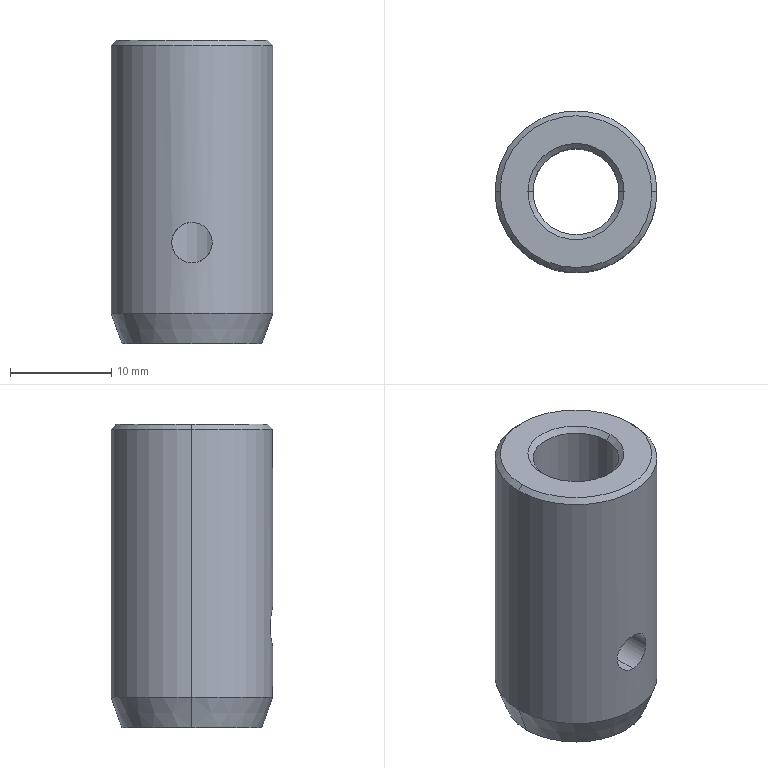Part | STEP file | 101000007764 | 1 solid | 16 faces | box 16 x 16 x 30 mm | volume 4190 mm3 | cone 8 | cylinder 6 | plane 2 | commonest cylinder face diameters 4 x2 8.5 x2 16 x2
STEP:
#1=CARTESIAN_POINT('',(0.,-8.,8.));
#2=VERTEX_POINT('',#1);
#3=CARTESIAN_POINT('',(0.,-8.,12.));
#4=VERTEX_POINT('',#3);
#5=CARTESIAN_POINT('',(0.,-8.,8.));
#6=CARTESIAN_POINT('',(-0.2045,-8.,8.));
#7=CARTESIAN_POINT('',(-0.4089,-7.993,8.026));
#8=CARTESIAN_POINT('',(-0.612,-7.98,8.079));
#9=CARTESIAN_POINT('',(-0.9324,-7.949,8.21));
#10=CARTESIAN_POINT('',(-1.216,-7.908,8.403));
#11=CARTESIAN_POINT('',(-1.323,-7.891,8.49));
#12=CARTESIAN_POINT('',(-1.666,-7.83,8.824));
#13=CARTESIAN_POINT('',(-1.902,-7.773,9.252));
#14=CARTESIAN_POINT('',(-2.003,-7.744,9.593));
#15=CARTESIAN_POINT('',(-2.038,-7.736,10.08));
#16=CARTESIAN_POINT('',(-1.931,-7.764,10.548));
#17=CARTESIAN_POINT('',(-1.888,-7.774,10.68));
#18=CARTESIAN_POINT('',(-1.728,-7.813,11.062));
#19=CARTESIAN_POINT('',(-1.474,-7.866,11.393));
#20=CARTESIAN_POINT('',(-1.269,-7.903,11.583));
#21=CARTESIAN_POINT('',(-0.8981,-7.956,11.822));
#22=CARTESIAN_POINT('',(-0.4782,-7.988,11.952));
#23=CARTESIAN_POINT('',(-0.3213,-7.996,11.984));
#24=CARTESIAN_POINT('',(-0.161,-8.,12.));
#25=CARTESIAN_POINT('',(0.,-8.,12.));
#26=B_SPLINE_CURVE_WITH_KNOTS('',5,(#5,#6,#7,#8,#9,#10,#11,#12,#13,#14,#15,#16,#17,#18,#19,#20,#21,#22,#23,#24,#25),.UNSPECIFIED.,.F.,.U.,(6,3,3,3,3,3,6),(0.,1.45,2.436,4.857,5.828,7.793,8.929),.UNSPECIFIED.);
#27=EDGE_CURVE('',#2,#4,#26,.T.);
#28=ORIENTED_EDGE('',*,*,#27,.F.);
#29=CARTESIAN_POINT('',(0.,-4.25,8.));
#30=VERTEX_POINT('',#29);
#31=CARTESIAN_POINT('',(0.,-22.,8.));
#32=DIRECTION('',(0.,1.,0.));
#33=VECTOR('',#32,1.);
#34=LINE('',#31,#33);
#35=EDGE_CURVE('',#2,#30,#34,.T.);
#36=ORIENTED_EDGE('',*,*,#35,.T.);
#37=CARTESIAN_POINT('',(0.,-4.25,12.));
#38=VERTEX_POINT('',#37);
#39=CARTESIAN_POINT('',(0.,-4.25,12.));
#40=CARTESIAN_POINT('',(-0.1332,-4.25,12.));
#41=CARTESIAN_POINT('',(-0.2653,-4.245,11.989));
#42=CARTESIAN_POINT('',(-0.3957,-4.234,11.967));
#43=CARTESIAN_POINT('',(-0.6561,-4.204,11.901));
#44=CARTESIAN_POINT('',(-0.8999,-4.157,11.794));
#45=CARTESIAN_POINT('',(-1.02,-4.128,11.728));
#46=CARTESIAN_POINT('',(-1.411,-4.022,11.47));
#47=CARTESIAN_POINT('',(-1.714,-3.898,11.109));
#48=CARTESIAN_POINT('',(-1.877,-3.815,10.808));
#49=CARTESIAN_POINT('',(-2.009,-3.745,10.349));
#50=CARTESIAN_POINT('',(-2.003,-3.749,9.875));
#51=CARTESIAN_POINT('',(-1.99,-3.756,9.741));
#52=CARTESIAN_POINT('',(-1.93,-3.787,9.41));
#53=CARTESIAN_POINT('',(-1.804,-3.85,9.101));
#54=CARTESIAN_POINT('',(-1.704,-3.896,8.924));
#55=CARTESIAN_POINT('',(-1.464,-3.997,8.601));
#56=CARTESIAN_POINT('',(-1.152,-4.096,8.347));
#57=CARTESIAN_POINT('',(-0.972,-4.144,8.235));
#58=CARTESIAN_POINT('',(-0.6779,-4.203,8.1));
#59=CARTESIAN_POINT('',(-0.3611,-4.237,8.027));
#60=CARTESIAN_POINT('',(-0.2413,-4.245,8.009));
#61=CARTESIAN_POINT('',(-0.1207,-4.25,8.));
#62=CARTESIAN_POINT('',(0.,-4.25,8.));
#63=B_SPLINE_CURVE_WITH_KNOTS('',5,(#39,#40,#41,#42,#43,#44,#45,#46,#47,#48,#49,#50,#51,#52,#53,#54,#55,#56,#57,#58,#59,#60,#61,#62),.UNSPECIFIED.,.F.,.U.,(6,3,3,3,3,3,3,6),(0.,0.9389,1.906,4.328,5.251,6.71,8.164,9.019),.UNSPECIFIED.);
#64=EDGE_CURVE('',#38,#30,#63,.T.);
#65=ORIENTED_EDGE('',*,*,#64,.F.);
#66=CARTESIAN_POINT('',(0.,-22.,12.));
#67=DIRECTION('',(0.,1.,0.));
#68=VECTOR('',#67,1.);
#69=LINE('',#66,#68);
#70=EDGE_CURVE('',#4,#38,#69,.T.);
#71=ORIENTED_EDGE('',*,*,#70,.F.);
#72=EDGE_LOOP('',(#28,#36,#65,#71));
#73=FACE_OUTER_BOUND('',#72,.T.);
#74=CARTESIAN_POINT('',(0.,-22.,10.));
#75=DIRECTION('',(0.,1.,0.));
#76=DIRECTION('',(0.,0.,-1.));
#77=AXIS2_PLACEMENT_3D('',#74,#75,#76);
#78=CYLINDRICAL_SURFACE('',#77,2.);
#79=ADVANCED_FACE('',(#73),#78,.F.);
#80=CARTESIAN_POINT('',(8.,0.,29.5));
#81=VERTEX_POINT('',#80);
#82=CARTESIAN_POINT('',(8.,0.,3.));
#83=VERTEX_POINT('',#82);
#84=CARTESIAN_POINT('',(8.,0.,30.));
#85=DIRECTION('',(0.,0.,-1.));
#86=VECTOR('',#85,1.);
#87=LINE('',#84,#86);
#88=EDGE_CURVE('',#81,#83,#87,.T.);
#89=ORIENTED_EDGE('',*,*,#88,.F.);
#90=CARTESIAN_POINT('',(-8.,0.,29.5));
#91=VERTEX_POINT('',#90);
#92=CARTESIAN_POINT('',(0.,0.,29.5));
#93=DIRECTION('',(0.,0.,-1.));
#94=AXIS2_PLACEMENT_3D('',#92,#93,$);
#95=CIRCLE('',#94,8.);
#96=EDGE_CURVE('',#81,#91,#95,.T.);
#97=ORIENTED_EDGE('',*,*,#96,.T.);
#98=CARTESIAN_POINT('',(-8.,0.,3.));
#99=VERTEX_POINT('',#98);
#100=CARTESIAN_POINT('',(-8.,0.,30.));
#101=DIRECTION('',(0.,0.,-1.));
#102=VECTOR('',#101,1.);
#103=LINE('',#100,#102);
#104=EDGE_CURVE('',#91,#99,#103,.T.);
#105=ORIENTED_EDGE('',*,*,#104,.T.);
#106=CARTESIAN_POINT('',(0.,0.,3.));
#107=DIRECTION('',(0.,0.,-1.));
#108=AXIS2_PLACEMENT_3D('',#106,#107,$);
#109=CIRCLE('',#108,8.);
#110=EDGE_CURVE('',#99,#83,#109,.F.);
#111=ORIENTED_EDGE('',*,*,#110,.T.);
#112=EDGE_LOOP('',(#89,#97,#105,#111));
#113=FACE_OUTER_BOUND('',#112,.T.);
#114=CARTESIAN_POINT('',(0.,-8.,12.));
#115=CARTESIAN_POINT('',(0.1371,-8.,12.));
#116=CARTESIAN_POINT('',(0.2729,-7.997,11.989));
#117=CARTESIAN_POINT('',(0.4075,-7.991,11.965));
#118=CARTESIAN_POINT('',(0.6743,-7.974,11.895));
#119=CARTESIAN_POINT('',(0.9243,-7.948,11.782));
#120=CARTESIAN_POINT('',(1.044,-7.933,11.714));
#121=CARTESIAN_POINT('',(1.441,-7.876,11.443));
#122=CARTESIAN_POINT('',(1.748,-7.811,11.061));
#123=CARTESIAN_POINT('',(1.905,-7.77,10.742));
#124=CARTESIAN_POINT('',(2.023,-7.74,10.267));
#125=CARTESIAN_POINT('',(1.995,-7.747,9.785));
#126=CARTESIAN_POINT('',(1.976,-7.752,9.648));
#127=CARTESIAN_POINT('',(1.899,-7.772,9.313));
#128=CARTESIAN_POINT('',(1.752,-7.807,9.002));
#129=CARTESIAN_POINT('',(1.637,-7.832,8.824));
#130=CARTESIAN_POINT('',(1.415,-7.877,8.56));
#131=CARTESIAN_POINT('',(1.143,-7.919,8.35));
#132=CARTESIAN_POINT('',(1.026,-7.935,8.275));
#133=CARTESIAN_POINT('',(0.7623,-7.967,8.136));
#134=CARTESIAN_POINT('',(0.4779,-7.988,8.048));
#135=CARTESIAN_POINT('',(0.32,-7.996,8.016));
#136=CARTESIAN_POINT('',(0.1594,-8.,8.));
#137=CARTESIAN_POINT('',(0.,-8.,8.));
#138=B_SPLINE_CURVE_WITH_KNOTS('',5,(#114,#115,#116,#117,#118,#119,#120,#121,#122,#123,#124,#125,#126,#127,#128,#129,#130,#131,#132,#133,#134,#135,#136,#137),.UNSPECIFIED.,.F.,.U.,(6,3,3,3,3,3,3,6),(0.,0.9654,1.944,4.382,5.348,6.812,7.793,8.924),.UNSPECIFIED.);
#139=EDGE_CURVE('',#4,#2,#138,.T.);
#140=ORIENTED_EDGE('',*,*,#139,.T.);
#141=ORIENTED_EDGE('',*,*,#27,.T.);
#142=EDGE_LOOP('',(#140,#141));
#143=FACE_BOUND('',#142,.T.);
#144=CARTESIAN_POINT('',(0.,0.,30.));
#145=DIRECTION('',(0.,0.,-1.));
#146=DIRECTION('',(1.,0.,0.));
#147=AXIS2_PLACEMENT_3D('',#144,#145,#146);
#148=CYLINDRICAL_SURFACE('',#147,8.);
#149=ADVANCED_FACE('',(#113,#143),#148,.T.);
#150=ORIENTED_EDGE('',*,*,#35,.F.);
#151=ORIENTED_EDGE('',*,*,#139,.F.);
#152=ORIENTED_EDGE('',*,*,#70,.T.);
#153=CARTESIAN_POINT('',(0.,-4.25,8.));
#154=CARTESIAN_POINT('',(0.132,-4.25,8.));
#155=CARTESIAN_POINT('',(0.2645,-4.245,8.011));
#156=CARTESIAN_POINT('',(0.3941,-4.235,8.033));
#157=CARTESIAN_POINT('',(0.7228,-4.196,8.116));
#158=CARTESIAN_POINT('',(1.025,-4.131,8.264));
#159=CARTESIAN_POINT('',(1.197,-4.083,8.378));
#160=CARTESIAN_POINT('',(1.403,-4.015,8.556));
#161=CARTESIAN_POINT('',(1.575,-3.948,8.764));
#162=CARTESIAN_POINT('',(1.616,-3.931,8.819));
#163=CARTESIAN_POINT('',(1.73,-3.883,8.984));
#164=CARTESIAN_POINT('',(1.824,-3.839,9.164));
#165=CARTESIAN_POINT('',(1.875,-3.815,9.284));
#166=CARTESIAN_POINT('',(1.956,-3.773,9.534));
#167=CARTESIAN_POINT('',(1.996,-3.752,9.797));
#168=CARTESIAN_POINT('',(2.005,-3.747,9.929));
#169=CARTESIAN_POINT('',(2.001,-3.75,10.262));
#170=CARTESIAN_POINT('',(1.928,-3.788,10.586));
#171=CARTESIAN_POINT('',(1.86,-3.823,10.775));
#172=CARTESIAN_POINT('',(1.736,-3.882,11.019));
#173=CARTESIAN_POINT('',(1.575,-3.948,11.236));
#174=CARTESIAN_POINT('',(1.532,-3.964,11.288));
#175=CARTESIAN_POINT('',(1.449,-3.996,11.382));
#176=CARTESIAN_POINT('',(1.359,-4.027,11.47));
#177=CARTESIAN_POINT('',(1.309,-4.044,11.515));
#178=CARTESIAN_POINT('',(1.149,-4.094,11.646));
#179=CARTESIAN_POINT('',(0.9715,-4.14,11.756));
#180=CARTESIAN_POINT('',(0.8498,-4.167,11.818));
#181=CARTESIAN_POINT('',(0.614,-4.21,11.914));
#182=CARTESIAN_POINT('',(0.364,-4.237,11.972));
#183=CARTESIAN_POINT('',(0.2441,-4.246,11.991));
#184=CARTESIAN_POINT('',(0.1221,-4.25,12.));
#185=CARTESIAN_POINT('',(0.,-4.25,12.));
#186=B_SPLINE_CURVE_WITH_KNOTS('',5,(#153,#154,#155,#156,#157,#158,#159,#160,#161,#162,#163,#164,#165,#166,#167,#168,#169,#170,#171,#172,#173,#174,#175,#176,#177,#178,#179,#180,#181,#182,#183,#184,#185),.UNSPECIFIED.,.F.,.U.,(6,3,3,3,3,3,3,3,3,3,6),(0.,0.9358,2.408,2.909,3.868,4.791,6.213,6.756,7.298,8.265,9.125),.UNSPECIFIED.);
#187=EDGE_CURVE('',#30,#38,#186,.T.);
#188=ORIENTED_EDGE('',*,*,#187,.F.);
#189=EDGE_LOOP('',(#150,#151,#152,#188));
#190=FACE_OUTER_BOUND('',#189,.T.);
#191=CARTESIAN_POINT('',(0.,-22.,10.));
#192=DIRECTION('',(0.,1.,0.));
#193=DIRECTION('',(0.,0.,1.));
#194=AXIS2_PLACEMENT_3D('',#191,#192,#193);
#195=CYLINDRICAL_SURFACE('',#194,2.);
#196=ADVANCED_FACE('',(#190),#195,.F.);
#197=CARTESIAN_POINT('',(4.25,0.,0.5));
#198=VERTEX_POINT('',#197);
#199=CARTESIAN_POINT('',(-4.25,0.,0.5));
#200=VERTEX_POINT('',#199);
#201=CARTESIAN_POINT('',(0.,0.,0.5));
#202=DIRECTION('',(0.,0.,1.));
#203=AXIS2_PLACEMENT_3D('',#201,#202,$);
#204=CIRCLE('',#203,4.25);
#205=EDGE_CURVE('',#198,#200,#204,.F.);
#206=ORIENTED_EDGE('',*,*,#205,.T.);
#207=CARTESIAN_POINT('',(-4.25,0.,29.5));
#208=VERTEX_POINT('',#207);
#209=CARTESIAN_POINT('',(-4.25,0.,30.));
#210=DIRECTION('',(0.,0.,1.));
#211=VECTOR('',#210,1.);
#212=LINE('',#209,#211);
#213=EDGE_CURVE('',#200,#208,#212,.T.);
#214=ORIENTED_EDGE('',*,*,#213,.T.);
#215=CARTESIAN_POINT('',(4.25,0.,29.5));
#216=VERTEX_POINT('',#215);
#217=CARTESIAN_POINT('',(0.,0.,29.5));
#218=DIRECTION('',(0.,0.,1.));
#219=AXIS2_PLACEMENT_3D('',#217,#218,$);
#220=CIRCLE('',#219,4.25);
#221=EDGE_CURVE('',#208,#216,#220,.T.);
#222=ORIENTED_EDGE('',*,*,#221,.T.);
#223=CARTESIAN_POINT('',(4.25,0.,30.));
#224=DIRECTION('',(0.,0.,1.));
#225=VECTOR('',#224,1.);
#226=LINE('',#223,#225);
#227=EDGE_CURVE('',#198,#216,#226,.T.);
#228=ORIENTED_EDGE('',*,*,#227,.F.);
#229=EDGE_LOOP('',(#206,#214,#222,#228));
#230=FACE_OUTER_BOUND('',#229,.T.);
#231=ORIENTED_EDGE('',*,*,#64,.T.);
#232=ORIENTED_EDGE('',*,*,#187,.T.);
#233=EDGE_LOOP('',(#231,#232));
#234=FACE_BOUND('',#233,.T.);
#235=CARTESIAN_POINT('',(0.,0.,30.));
#236=DIRECTION('',(0.,0.,1.));
#237=DIRECTION('',(-1.,0.,0.));
#238=AXIS2_PLACEMENT_3D('',#235,#236,#237);
#239=CYLINDRICAL_SURFACE('',#238,4.25);
#240=ADVANCED_FACE('',(#230,#234),#239,.F.);
#241=CARTESIAN_POINT('',(0.,0.,29.5));
#242=DIRECTION('',(0.,0.,-1.));
#243=AXIS2_PLACEMENT_3D('',#241,#242,$);
#244=CIRCLE('',#243,8.);
#245=EDGE_CURVE('',#91,#81,#244,.T.);
#246=ORIENTED_EDGE('',*,*,#245,.T.);
#247=ORIENTED_EDGE('',*,*,#88,.T.);
#248=CARTESIAN_POINT('',(0.,0.,3.));
#249=DIRECTION('',(0.,0.,-1.));
#250=AXIS2_PLACEMENT_3D('',#248,#249,$);
#251=CIRCLE('',#250,8.);
#252=EDGE_CURVE('',#83,#99,#251,.F.);
#253=ORIENTED_EDGE('',*,*,#252,.T.);
#254=ORIENTED_EDGE('',*,*,#104,.F.);
#255=EDGE_LOOP('',(#246,#247,#253,#254));
#256=FACE_OUTER_BOUND('',#255,.T.);
#257=CARTESIAN_POINT('',(0.,0.,30.));
#258=DIRECTION('',(0.,0.,-1.));
#259=DIRECTION('',(-1.,0.,0.));
#260=AXIS2_PLACEMENT_3D('',#257,#258,#259);
#261=CYLINDRICAL_SURFACE('',#260,8.);
#262=ADVANCED_FACE('',(#256),#261,.T.);
#263=CARTESIAN_POINT('',(7.5,0.,30.));
#264=VERTEX_POINT('',#263);
#265=CARTESIAN_POINT('',(353557.141,0.,-353519.641));
#266=DIRECTION('',(0.7071,0.,-0.7071));
#267=VECTOR('',#266,1.);
#268=LINE('',#265,#267);
#269=EDGE_CURVE('',#264,#81,#268,.T.);
#270=ORIENTED_EDGE('',*,*,#269,.F.);
#271=CARTESIAN_POINT('',(-7.5,0.,30.));
#272=VERTEX_POINT('',#271);
#273=CARTESIAN_POINT('',(0.,0.,30.));
#274=DIRECTION('',(0.,0.,-1.));
#275=AXIS2_PLACEMENT_3D('',#273,#274,$);
#276=CIRCLE('',#275,7.5);
#277=EDGE_CURVE('',#272,#264,#276,.F.);
#278=ORIENTED_EDGE('',*,*,#277,.F.);
#279=CARTESIAN_POINT('',(-353557.141,0.,-353519.641));
#280=DIRECTION('',(-0.7071,0.,-0.7071));
#281=VECTOR('',#280,1.);
#282=LINE('',#279,#281);
#283=EDGE_CURVE('',#272,#91,#282,.T.);
#284=ORIENTED_EDGE('',*,*,#283,.T.);
#285=ORIENTED_EDGE('',*,*,#96,.F.);
#286=EDGE_LOOP('',(#270,#278,#284,#285));
#287=FACE_OUTER_BOUND('',#286,.T.);
#288=CARTESIAN_POINT('',(0.,0.,30.));
#289=DIRECTION('',(0.,0.,-1.));
#290=DIRECTION('',(1.,0.,0.));
#291=AXIS2_PLACEMENT_3D('',#288,#289,#290);
#292=CONICAL_SURFACE('',#291,7.5,0.7854);
#293=ADVANCED_FACE('',(#287),#292,.T.);
#294=CARTESIAN_POINT('',(-6.908,0.,0.));
#295=VERTEX_POINT('',#294);
#296=CARTESIAN_POINT('',(-171014.072,0.,469838.32));
#297=DIRECTION('',(-0.342,0.,0.9397));
#298=VECTOR('',#297,1.);
#299=LINE('',#296,#298);
#300=EDGE_CURVE('',#295,#99,#299,.T.);
#301=ORIENTED_EDGE('',*,*,#300,.F.);
#302=CARTESIAN_POINT('',(6.908,0.,0.));
#303=VERTEX_POINT('',#302);
#304=CARTESIAN_POINT('',(0.,0.,0.));
#305=DIRECTION('',(0.,0.,1.));
#306=AXIS2_PLACEMENT_3D('',#304,#305,$);
#307=CIRCLE('',#306,6.908);
#308=EDGE_CURVE('',#303,#295,#307,.F.);
#309=ORIENTED_EDGE('',*,*,#308,.F.);
#310=CARTESIAN_POINT('',(171014.072,0.,469838.32));
#311=DIRECTION('',(0.342,0.,0.9397));
#312=VECTOR('',#311,1.);
#313=LINE('',#310,#312);
#314=EDGE_CURVE('',#303,#83,#313,.T.);
#315=ORIENTED_EDGE('',*,*,#314,.T.);
#316=ORIENTED_EDGE('',*,*,#110,.F.);
#317=EDGE_LOOP('',(#301,#309,#315,#316));
#318=FACE_OUTER_BOUND('',#317,.T.);
#319=CARTESIAN_POINT('',(0.,0.,3.));
#320=DIRECTION('',(0.,0.,1.));
#321=DIRECTION('',(-1.,0.,0.));
#322=AXIS2_PLACEMENT_3D('',#319,#320,#321);
#323=CONICAL_SURFACE('',#322,8.,0.3491);
#324=ADVANCED_FACE('',(#318),#323,.T.);
#325=ORIENTED_EDGE('',*,*,#205,.F.);
#326=CARTESIAN_POINT('',(4.75,0.,0.));
#327=VERTEX_POINT('',#326);
#328=CARTESIAN_POINT('',(353555.766,0.,-353551.016));
#329=DIRECTION('',(0.7071,0.,-0.7071));
#330=VECTOR('',#329,1.);
#331=LINE('',#328,#330);
#332=EDGE_CURVE('',#198,#327,#331,.T.);
#333=ORIENTED_EDGE('',*,*,#332,.T.);
#334=CARTESIAN_POINT('',(-4.75,0.,0.));
#335=VERTEX_POINT('',#334);
#336=CARTESIAN_POINT('',(0.,0.,0.));
#337=DIRECTION('',(0.,0.,-1.));
#338=AXIS2_PLACEMENT_3D('',#336,#337,$);
#339=CIRCLE('',#338,4.75);
#340=EDGE_CURVE('',#335,#327,#339,.F.);
#341=ORIENTED_EDGE('',*,*,#340,.F.);
#342=CARTESIAN_POINT('',(-353555.766,0.,-353551.016));
#343=DIRECTION('',(-0.7071,0.,-0.7071));
#344=VECTOR('',#343,1.);
#345=LINE('',#342,#344);
#346=EDGE_CURVE('',#200,#335,#345,.T.);
#347=ORIENTED_EDGE('',*,*,#346,.F.);
#348=EDGE_LOOP('',(#325,#333,#341,#347));
#349=FACE_OUTER_BOUND('',#348,.T.);
#350=CARTESIAN_POINT('',(0.,0.,0.));
#351=DIRECTION('',(0.,0.,-1.));
#352=DIRECTION('',(1.,0.,0.));
#353=AXIS2_PLACEMENT_3D('',#350,#351,#352);
#354=CONICAL_SURFACE('',#353,4.75,0.7854);
#355=ADVANCED_FACE('',(#349),#354,.F.);
#356=ORIENTED_EDGE('',*,*,#213,.F.);
#357=CARTESIAN_POINT('',(0.,0.,0.5));
#358=DIRECTION('',(0.,0.,1.));
#359=AXIS2_PLACEMENT_3D('',#357,#358,$);
#360=CIRCLE('',#359,4.25);
#361=EDGE_CURVE('',#200,#198,#360,.F.);
#362=ORIENTED_EDGE('',*,*,#361,.T.);
#363=ORIENTED_EDGE('',*,*,#227,.T.);
#364=CARTESIAN_POINT('',(0.,0.,29.5));
#365=DIRECTION('',(0.,0.,1.));
#366=AXIS2_PLACEMENT_3D('',#364,#365,$);
#367=CIRCLE('',#366,4.25);
#368=EDGE_CURVE('',#216,#208,#367,.T.);
#369=ORIENTED_EDGE('',*,*,#368,.T.);
#370=EDGE_LOOP('',(#356,#362,#363,#369));
#371=FACE_OUTER_BOUND('',#370,.T.);
#372=CARTESIAN_POINT('',(0.,0.,30.));
#373=DIRECTION('',(0.,0.,1.));
#374=DIRECTION('',(1.,0.,0.));
#375=AXIS2_PLACEMENT_3D('',#372,#373,#374);
#376=CYLINDRICAL_SURFACE('',#375,4.25);
#377=ADVANCED_FACE('',(#371),#376,.F.);
#378=ORIENTED_EDGE('',*,*,#221,.F.);
#379=CARTESIAN_POINT('',(-4.75,0.,30.));
#380=VERTEX_POINT('',#379);
#381=CARTESIAN_POINT('',(-353555.516,0.,353580.766));
#382=DIRECTION('',(-0.7071,0.,0.7071));
#383=VECTOR('',#382,1.);
#384=LINE('',#381,#383);
#385=EDGE_CURVE('',#208,#380,#384,.T.);
#386=ORIENTED_EDGE('',*,*,#385,.T.);
#387=CARTESIAN_POINT('',(4.75,0.,30.));
#388=VERTEX_POINT('',#387);
#389=CARTESIAN_POINT('',(0.,0.,30.));
#390=DIRECTION('',(0.,0.,1.));
#391=AXIS2_PLACEMENT_3D('',#389,#390,$);
#392=CIRCLE('',#391,4.75);
#393=EDGE_CURVE('',#388,#380,#392,.F.);
#394=ORIENTED_EDGE('',*,*,#393,.F.);
#395=CARTESIAN_POINT('',(353555.516,0.,353580.766));
#396=DIRECTION('',(0.7071,0.,0.7071));
#397=VECTOR('',#396,1.);
#398=LINE('',#395,#397);
#399=EDGE_CURVE('',#216,#388,#398,.T.);
#400=ORIENTED_EDGE('',*,*,#399,.F.);
#401=EDGE_LOOP('',(#378,#386,#394,#400));
#402=FACE_OUTER_BOUND('',#401,.T.);
#403=CARTESIAN_POINT('',(0.,0.,29.5));
#404=DIRECTION('',(0.,0.,1.));
#405=DIRECTION('',(-1.,0.,0.));
#406=AXIS2_PLACEMENT_3D('',#403,#404,#405);
#407=CONICAL_SURFACE('',#406,4.25,0.7854);
#408=ADVANCED_FACE('',(#402),#407,.F.);
#409=CARTESIAN_POINT('',(0.,0.,30.));
#410=DIRECTION('',(0.,0.,-1.));
#411=AXIS2_PLACEMENT_3D('',#409,#410,$);
#412=CIRCLE('',#411,7.5);
#413=EDGE_CURVE('',#264,#272,#412,.F.);
#414=ORIENTED_EDGE('',*,*,#413,.F.);
#415=ORIENTED_EDGE('',*,*,#269,.T.);
#416=ORIENTED_EDGE('',*,*,#245,.F.);
#417=ORIENTED_EDGE('',*,*,#283,.F.);
#418=EDGE_LOOP('',(#414,#415,#416,#417));
#419=FACE_OUTER_BOUND('',#418,.T.);
#420=CARTESIAN_POINT('',(0.,0.,30.));
#421=DIRECTION('',(0.,0.,-1.));
#422=DIRECTION('',(-1.,0.,0.));
#423=AXIS2_PLACEMENT_3D('',#420,#421,#422);
#424=CONICAL_SURFACE('',#423,7.5,0.7854);
#425=ADVANCED_FACE('',(#419),#424,.T.);
#426=CARTESIAN_POINT('',(0.,0.,0.));
#427=DIRECTION('',(0.,0.,1.));
#428=AXIS2_PLACEMENT_3D('',#426,#427,$);
#429=CIRCLE('',#428,6.908);
#430=EDGE_CURVE('',#295,#303,#429,.F.);
#431=ORIENTED_EDGE('',*,*,#430,.F.);
#432=ORIENTED_EDGE('',*,*,#300,.T.);
#433=ORIENTED_EDGE('',*,*,#252,.F.);
#434=ORIENTED_EDGE('',*,*,#314,.F.);
#435=EDGE_LOOP('',(#431,#432,#433,#434));
#436=FACE_OUTER_BOUND('',#435,.T.);
#437=CARTESIAN_POINT('',(0.,0.,3.));
#438=DIRECTION('',(0.,0.,1.));
#439=DIRECTION('',(1.,0.,0.));
#440=AXIS2_PLACEMENT_3D('',#437,#438,#439);
#441=CONICAL_SURFACE('',#440,8.,0.3491);
#442=ADVANCED_FACE('',(#436),#441,.T.);
#443=ORIENTED_EDGE('',*,*,#277,.T.);
#444=ORIENTED_EDGE('',*,*,#413,.T.);
#445=EDGE_LOOP('',(#443,#444));
#446=FACE_OUTER_BOUND('',#445,.T.);
#447=ORIENTED_EDGE('',*,*,#393,.T.);
#448=CARTESIAN_POINT('',(-4.75,0.,30.));
#449=CARTESIAN_POINT('',(-4.75,0.5338,30.));
#450=CARTESIAN_POINT('',(-4.675,1.068,30.));
#451=CARTESIAN_POINT('',(-4.525,1.588,30.));
#452=CARTESIAN_POINT('',(-4.083,2.571,30.));
#453=CARTESIAN_POINT('',(-3.387,3.395,30.));
#454=CARTESIAN_POINT('',(-2.983,3.754,30.));
#455=CARTESIAN_POINT('',(-2.085,4.351,30.));
#456=CARTESIAN_POINT('',(-1.058,4.677,30.));
#457=CARTESIAN_POINT('',(-0.5239,4.767,30.));
#458=CARTESIAN_POINT('',(0.5539,4.793,30.));
#459=CARTESIAN_POINT('',(1.597,4.522,30.));
#460=CARTESIAN_POINT('',(2.097,4.313,30.));
#461=CARTESIAN_POINT('',(3.023,3.761,30.));
#462=CARTESIAN_POINT('',(3.761,2.975,30.));
#463=CARTESIAN_POINT('',(4.072,2.532,30.));
#464=CARTESIAN_POINT('',(4.462,1.769,30.));
#465=CARTESIAN_POINT('',(4.672,0.9428,30.));
#466=CARTESIAN_POINT('',(4.724,0.6305,30.));
#467=CARTESIAN_POINT('',(4.75,0.3152,30.));
#468=CARTESIAN_POINT('',(4.75,0.,30.));
#469=B_SPLINE_CURVE_WITH_KNOTS('',5,(#448,#449,#450,#451,#452,#453,#454,#455,#456,#457,#458,#459,#460,#461,#462,#463,#464,#465,#466,#467,#468),.UNSPECIFIED.,.F.,.U.,(6,3,3,3,3,3,6),(0.,3.775,7.55,11.325,15.099,18.874,21.103),.UNSPECIFIED.);
#470=EDGE_CURVE('',#380,#388,#469,.T.);
#471=ORIENTED_EDGE('',*,*,#470,.T.);
#472=EDGE_LOOP('',(#447,#471));
#473=FACE_BOUND('',#472,.T.);
#474=CARTESIAN_POINT('',(0.,0.,30.));
#475=DIRECTION('',(0.,0.,1.));
#476=DIRECTION('',(1.,0.,0.));
#477=AXIS2_PLACEMENT_3D('',#474,#475,#476);
#478=PLANE('',#477);
#479=ADVANCED_FACE('',(#446,#473),#478,.T.);
#480=ORIENTED_EDGE('',*,*,#308,.T.);
#481=ORIENTED_EDGE('',*,*,#430,.T.);
#482=EDGE_LOOP('',(#480,#481));
#483=FACE_OUTER_BOUND('',#482,.T.);
#484=ORIENTED_EDGE('',*,*,#340,.T.);
#485=CARTESIAN_POINT('',(0.,0.,0.));
#486=DIRECTION('',(0.,0.,1.));
#487=AXIS2_PLACEMENT_3D('',#485,#486,$);
#488=CIRCLE('',#487,4.75);
#489=EDGE_CURVE('',#327,#335,#488,.T.);
#490=ORIENTED_EDGE('',*,*,#489,.T.);
#491=EDGE_LOOP('',(#484,#490));
#492=FACE_BOUND('',#491,.T.);
#493=CARTESIAN_POINT('',(0.,0.,0.));
#494=DIRECTION('',(0.,0.,1.));
#495=DIRECTION('',(1.,0.,0.));
#496=AXIS2_PLACEMENT_3D('',#493,#494,#495);
#497=PLANE('',#496);
#498=ADVANCED_FACE('',(#483,#492),#497,.F.);
#499=ORIENTED_EDGE('',*,*,#332,.F.);
#500=ORIENTED_EDGE('',*,*,#361,.F.);
#501=ORIENTED_EDGE('',*,*,#346,.T.);
#502=ORIENTED_EDGE('',*,*,#489,.F.);
#503=EDGE_LOOP('',(#499,#500,#501,#502));
#504=FACE_OUTER_BOUND('',#503,.T.);
#505=CARTESIAN_POINT('',(0.,0.,0.));
#506=DIRECTION('',(0.,0.,-1.));
#507=DIRECTION('',(-1.,0.,0.));
#508=AXIS2_PLACEMENT_3D('',#505,#506,#507);
#509=CONICAL_SURFACE('',#508,4.75,0.7854);
#510=ADVANCED_FACE('',(#504),#509,.F.);
#511=ORIENTED_EDGE('',*,*,#385,.F.);
#512=ORIENTED_EDGE('',*,*,#368,.F.);
#513=ORIENTED_EDGE('',*,*,#399,.T.);
#514=ORIENTED_EDGE('',*,*,#470,.F.);
#515=EDGE_LOOP('',(#511,#512,#513,#514));
#516=FACE_OUTER_BOUND('',#515,.T.);
#517=CARTESIAN_POINT('',(0.,0.,29.5));
#518=DIRECTION('',(0.,0.,1.));
#519=DIRECTION('',(1.,0.,0.));
#520=AXIS2_PLACEMENT_3D('',#517,#518,#519);
#521=CONICAL_SURFACE('',#520,4.25,0.7854);
#522=ADVANCED_FACE('',(#516),#521,.F.);
#523=CLOSED_SHELL('',(#79,#149,#196,#240,#262,#293,#324,#355,#377,#408,#425,#442,#479,#498,#510,#522));
#524=MANIFOLD_SOLID_BREP('',#523);
#525=(LENGTH_UNIT()NAMED_UNIT(*)SI_UNIT(.MILLI.,.METRE.));
#526=UNCERTAINTY_MEASURE_WITH_UNIT(LENGTH_MEASURE(0.005),#525,'','');
#527=(NAMED_UNIT(*)PLANE_ANGLE_UNIT()SI_UNIT($,.RADIAN.));
#528=(NAMED_UNIT(*)SI_UNIT($,.STERADIAN.)SOLID_ANGLE_UNIT());
#529=(GEOMETRIC_REPRESENTATION_CONTEXT(3)GLOBAL_UNCERTAINTY_ASSIGNED_CONTEXT((#526))GLOBAL_UNIT_ASSIGNED_CONTEXT((#525,#527,#528))REPRESENTATION_CONTEXT('',''));
#530=ADVANCED_BREP_SHAPE_REPRESENTATION('',(#524),#529);